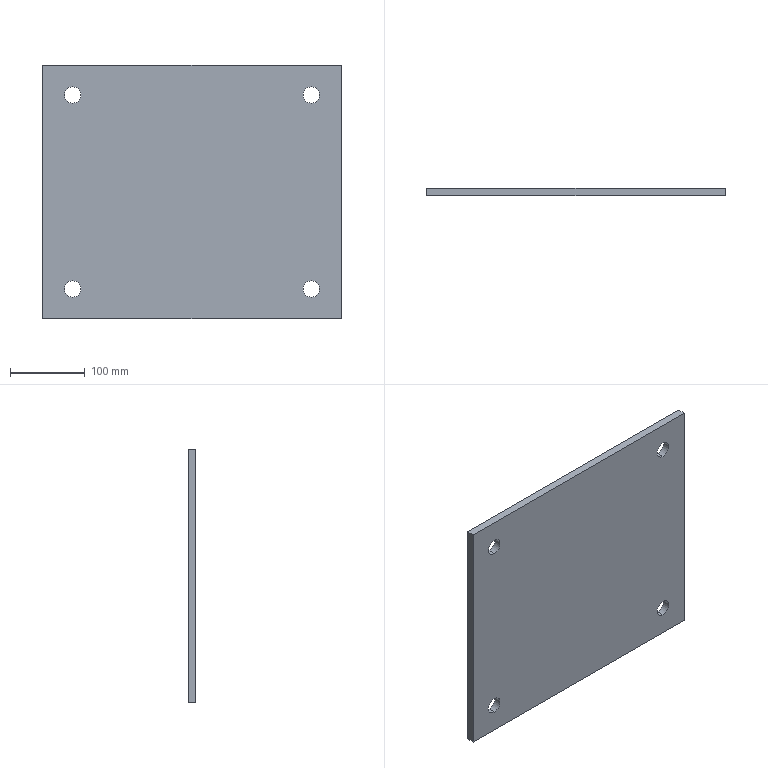Part | STEP file | 立柱Pad-中转釜 | 1 solid | 14 faces | box 400 x 10 x 340 mm | volume 1344795 mm3 | cylinder 8 | plane 6 | commonest cylinder face diameters 22 x8
STEP:
#1=CARTESIAN_POINT('',(0.,0.,0.));
#2=DIRECTION('',(0.,0.,1.));
#3=DIRECTION('',(1.,0.,0.));
#4=AXIS2_PLACEMENT_3D('',#1,#2,#3);
#5=CARTESIAN_POINT('',(160.,0.,-119.));
#6=VERTEX_POINT('',#5);
#7=CARTESIAN_POINT('',(160.,10.,-119.));
#8=VERTEX_POINT('',#7);
#9=CARTESIAN_POINT('',(160.,10.,-119.));
#10=DIRECTION('',(0.,1.,0.));
#11=VECTOR('',#10,1.);
#12=LINE('',#9,#11);
#13=CARTESIAN_POINT('',(160.,10.,-130.));
#14=DIRECTION('',(0.,1.,0.));
#15=DIRECTION('',(0.,0.,1.));
#16=AXIS2_PLACEMENT_3D('',#13,#14,#15);
#17=CYLINDRICAL_SURFACE('',#16,11.);
#18=CARTESIAN_POINT('',(6.283,0.));
#19=DIRECTION('',(0.,1.));
#20=VECTOR('',#19,1.);
#21=LINE('',#18,#20);
#22=(GEOMETRIC_REPRESENTATION_CONTEXT(2)PARAMETRIC_REPRESENTATION_CONTEXT()REPRESENTATION_CONTEXT('',''));
#23=DEFINITIONAL_REPRESENTATION('',(#21),#22);
#24=PCURVE('',#17,#23);
#25=CARTESIAN_POINT('',(160.,10.,-130.));
#26=DIRECTION('',(0.,1.,0.));
#27=DIRECTION('',(0.,0.,1.));
#28=AXIS2_PLACEMENT_3D('',#25,#26,#27);
#29=CYLINDRICAL_SURFACE('',#28,11.);
#30=CARTESIAN_POINT('',(0.,0.));
#31=DIRECTION('',(0.,1.));
#32=VECTOR('',#31,1.);
#33=LINE('',#30,#32);
#34=(GEOMETRIC_REPRESENTATION_CONTEXT(2)PARAMETRIC_REPRESENTATION_CONTEXT()REPRESENTATION_CONTEXT('',''));
#35=DEFINITIONAL_REPRESENTATION('',(#33),#34);
#36=PCURVE('',#29,#35);
#37=SURFACE_CURVE('',#12,(#24,#36),.PCURVE_S1.);
#38=EDGE_CURVE('',#6,#8,#37,.T.);
#39=ORIENTED_EDGE('',*,*,#38,.T.);
#40=CARTESIAN_POINT('',(160.,10.,-141.));
#41=VERTEX_POINT('',#40);
#42=CARTESIAN_POINT('',(160.,10.,-130.));
#43=DIRECTION('',(0.,1.,0.));
#44=DIRECTION('',(0.,0.,1.));
#45=AXIS2_PLACEMENT_3D('',#42,#43,#44);
#46=CIRCLE('',#45,11.);
#47=CARTESIAN_POINT('',(0.,0.));
#48=DIRECTION('',(1.,0.));
#49=VECTOR('',#48,1.);
#50=LINE('',#47,#49);
#51=(GEOMETRIC_REPRESENTATION_CONTEXT(2)PARAMETRIC_REPRESENTATION_CONTEXT()REPRESENTATION_CONTEXT('',''));
#52=DEFINITIONAL_REPRESENTATION('',(#50),#51);
#53=PCURVE('',#17,#52);
#54=CARTESIAN_POINT('',(0.,10.,0.));
#55=DIRECTION('',(0.,1.,0.));
#56=DIRECTION('',(0.,0.,1.));
#57=AXIS2_PLACEMENT_3D('',#54,#55,#56);
#58=PLANE('',#57);
#59=CARTESIAN_POINT('',(-130.,160.));
#60=DIRECTION('',(1.,0.));
#61=AXIS2_PLACEMENT_2D('',#59,#60);
#62=CIRCLE('',#61,11.);
#63=(GEOMETRIC_REPRESENTATION_CONTEXT(2)PARAMETRIC_REPRESENTATION_CONTEXT()REPRESENTATION_CONTEXT('',''));
#64=DEFINITIONAL_REPRESENTATION('',(#62),#63);
#65=PCURVE('',#58,#64);
#66=SURFACE_CURVE('',#46,(#53,#65),.PCURVE_S1.);
#67=EDGE_CURVE('',#41,#8,#66,.T.);
#68=ORIENTED_EDGE('',*,*,#67,.F.);
#69=CARTESIAN_POINT('',(160.,0.,-141.));
#70=VERTEX_POINT('',#69);
#71=CARTESIAN_POINT('',(160.,10.,-141.));
#72=DIRECTION('',(0.,1.,0.));
#73=VECTOR('',#72,1.);
#74=LINE('',#71,#73);
#75=CARTESIAN_POINT('',(3.142,0.));
#76=DIRECTION('',(0.,1.));
#77=VECTOR('',#76,1.);
#78=LINE('',#75,#77);
#79=(GEOMETRIC_REPRESENTATION_CONTEXT(2)PARAMETRIC_REPRESENTATION_CONTEXT()REPRESENTATION_CONTEXT('',''));
#80=DEFINITIONAL_REPRESENTATION('',(#78),#79);
#81=PCURVE('',#17,#80);
#82=CARTESIAN_POINT('',(3.142,0.));
#83=DIRECTION('',(0.,1.));
#84=VECTOR('',#83,1.);
#85=LINE('',#82,#84);
#86=(GEOMETRIC_REPRESENTATION_CONTEXT(2)PARAMETRIC_REPRESENTATION_CONTEXT()REPRESENTATION_CONTEXT('',''));
#87=DEFINITIONAL_REPRESENTATION('',(#85),#86);
#88=PCURVE('',#29,#87);
#89=SURFACE_CURVE('',#74,(#81,#88),.PCURVE_S1.);
#90=EDGE_CURVE('',#70,#41,#89,.T.);
#91=ORIENTED_EDGE('',*,*,#90,.F.);
#92=CARTESIAN_POINT('',(160.,0.,-130.));
#93=DIRECTION('',(0.,1.,0.));
#94=DIRECTION('',(0.,0.,1.));
#95=AXIS2_PLACEMENT_3D('',#92,#93,#94);
#96=CIRCLE('',#95,11.);
#97=CARTESIAN_POINT('',(0.,-10.));
#98=DIRECTION('',(1.,0.));
#99=VECTOR('',#98,1.);
#100=LINE('',#97,#99);
#101=(GEOMETRIC_REPRESENTATION_CONTEXT(2)PARAMETRIC_REPRESENTATION_CONTEXT()REPRESENTATION_CONTEXT('',''));
#102=DEFINITIONAL_REPRESENTATION('',(#100),#101);
#103=PCURVE('',#17,#102);
#104=CARTESIAN_POINT('',(0.,0.,0.));
#105=DIRECTION('',(0.,1.,0.));
#106=DIRECTION('',(0.,0.,1.));
#107=AXIS2_PLACEMENT_3D('',#104,#105,#106);
#108=PLANE('',#107);
#109=CARTESIAN_POINT('',(-130.,160.));
#110=DIRECTION('',(1.,0.));
#111=AXIS2_PLACEMENT_2D('',#109,#110);
#112=CIRCLE('',#111,11.);
#113=(GEOMETRIC_REPRESENTATION_CONTEXT(2)PARAMETRIC_REPRESENTATION_CONTEXT()REPRESENTATION_CONTEXT('',''));
#114=DEFINITIONAL_REPRESENTATION('',(#112),#113);
#115=PCURVE('',#108,#114);
#116=SURFACE_CURVE('',#96,(#103,#115),.PCURVE_S1.);
#117=EDGE_CURVE('',#70,#6,#116,.T.);
#118=ORIENTED_EDGE('',*,*,#117,.T.);
#119=EDGE_LOOP('',(#39,#68,#91,#118));
#120=FACE_BOUND('',#119,.F.);
#121=ADVANCED_FACE('',(#120),#17,.F.);
#122=CARTESIAN_POINT('',(160.,0.,141.));
#123=VERTEX_POINT('',#122);
#124=CARTESIAN_POINT('',(160.,10.,141.));
#125=VERTEX_POINT('',#124);
#126=CARTESIAN_POINT('',(160.,10.,141.));
#127=DIRECTION('',(0.,1.,0.));
#128=VECTOR('',#127,1.);
#129=LINE('',#126,#128);
#130=CARTESIAN_POINT('',(160.,10.,130.));
#131=DIRECTION('',(0.,1.,0.));
#132=DIRECTION('',(0.,0.,1.));
#133=AXIS2_PLACEMENT_3D('',#130,#131,#132);
#134=CYLINDRICAL_SURFACE('',#133,11.);
#135=CARTESIAN_POINT('',(6.283,0.));
#136=DIRECTION('',(0.,1.));
#137=VECTOR('',#136,1.);
#138=LINE('',#135,#137);
#139=(GEOMETRIC_REPRESENTATION_CONTEXT(2)PARAMETRIC_REPRESENTATION_CONTEXT()REPRESENTATION_CONTEXT('',''));
#140=DEFINITIONAL_REPRESENTATION('',(#138),#139);
#141=PCURVE('',#134,#140);
#142=CARTESIAN_POINT('',(160.,10.,130.));
#143=DIRECTION('',(0.,1.,0.));
#144=DIRECTION('',(0.,0.,1.));
#145=AXIS2_PLACEMENT_3D('',#142,#143,#144);
#146=CYLINDRICAL_SURFACE('',#145,11.);
#147=CARTESIAN_POINT('',(0.,0.));
#148=DIRECTION('',(0.,1.));
#149=VECTOR('',#148,1.);
#150=LINE('',#147,#149);
#151=(GEOMETRIC_REPRESENTATION_CONTEXT(2)PARAMETRIC_REPRESENTATION_CONTEXT()REPRESENTATION_CONTEXT('',''));
#152=DEFINITIONAL_REPRESENTATION('',(#150),#151);
#153=PCURVE('',#146,#152);
#154=SURFACE_CURVE('',#129,(#141,#153),.PCURVE_S1.);
#155=EDGE_CURVE('',#123,#125,#154,.T.);
#156=ORIENTED_EDGE('',*,*,#155,.T.);
#157=CARTESIAN_POINT('',(160.,10.,119.));
#158=VERTEX_POINT('',#157);
#159=CARTESIAN_POINT('',(160.,10.,130.));
#160=DIRECTION('',(0.,1.,0.));
#161=DIRECTION('',(0.,0.,1.));
#162=AXIS2_PLACEMENT_3D('',#159,#160,#161);
#163=CIRCLE('',#162,11.);
#164=CARTESIAN_POINT('',(0.,0.));
#165=DIRECTION('',(1.,0.));
#166=VECTOR('',#165,1.);
#167=LINE('',#164,#166);
#168=(GEOMETRIC_REPRESENTATION_CONTEXT(2)PARAMETRIC_REPRESENTATION_CONTEXT()REPRESENTATION_CONTEXT('',''));
#169=DEFINITIONAL_REPRESENTATION('',(#167),#168);
#170=PCURVE('',#134,#169);
#171=CARTESIAN_POINT('',(130.,160.));
#172=DIRECTION('',(1.,0.));
#173=AXIS2_PLACEMENT_2D('',#171,#172);
#174=CIRCLE('',#173,11.);
#175=(GEOMETRIC_REPRESENTATION_CONTEXT(2)PARAMETRIC_REPRESENTATION_CONTEXT()REPRESENTATION_CONTEXT('',''));
#176=DEFINITIONAL_REPRESENTATION('',(#174),#175);
#177=PCURVE('',#58,#176);
#178=SURFACE_CURVE('',#163,(#170,#177),.PCURVE_S1.);
#179=EDGE_CURVE('',#158,#125,#178,.T.);
#180=ORIENTED_EDGE('',*,*,#179,.F.);
#181=CARTESIAN_POINT('',(160.,0.,119.));
#182=VERTEX_POINT('',#181);
#183=CARTESIAN_POINT('',(160.,10.,119.));
#184=DIRECTION('',(0.,1.,0.));
#185=VECTOR('',#184,1.);
#186=LINE('',#183,#185);
#187=CARTESIAN_POINT('',(3.142,0.));
#188=DIRECTION('',(0.,1.));
#189=VECTOR('',#188,1.);
#190=LINE('',#187,#189);
#191=(GEOMETRIC_REPRESENTATION_CONTEXT(2)PARAMETRIC_REPRESENTATION_CONTEXT()REPRESENTATION_CONTEXT('',''));
#192=DEFINITIONAL_REPRESENTATION('',(#190),#191);
#193=PCURVE('',#134,#192);
#194=CARTESIAN_POINT('',(3.142,0.));
#195=DIRECTION('',(0.,1.));
#196=VECTOR('',#195,1.);
#197=LINE('',#194,#196);
#198=(GEOMETRIC_REPRESENTATION_CONTEXT(2)PARAMETRIC_REPRESENTATION_CONTEXT()REPRESENTATION_CONTEXT('',''));
#199=DEFINITIONAL_REPRESENTATION('',(#197),#198);
#200=PCURVE('',#146,#199);
#201=SURFACE_CURVE('',#186,(#193,#200),.PCURVE_S1.);
#202=EDGE_CURVE('',#182,#158,#201,.T.);
#203=ORIENTED_EDGE('',*,*,#202,.F.);
#204=CARTESIAN_POINT('',(160.,0.,130.));
#205=DIRECTION('',(0.,1.,0.));
#206=DIRECTION('',(0.,0.,1.));
#207=AXIS2_PLACEMENT_3D('',#204,#205,#206);
#208=CIRCLE('',#207,11.);
#209=CARTESIAN_POINT('',(0.,-10.));
#210=DIRECTION('',(1.,0.));
#211=VECTOR('',#210,1.);
#212=LINE('',#209,#211);
#213=(GEOMETRIC_REPRESENTATION_CONTEXT(2)PARAMETRIC_REPRESENTATION_CONTEXT()REPRESENTATION_CONTEXT('',''));
#214=DEFINITIONAL_REPRESENTATION('',(#212),#213);
#215=PCURVE('',#134,#214);
#216=CARTESIAN_POINT('',(130.,160.));
#217=DIRECTION('',(1.,0.));
#218=AXIS2_PLACEMENT_2D('',#216,#217);
#219=CIRCLE('',#218,11.);
#220=(GEOMETRIC_REPRESENTATION_CONTEXT(2)PARAMETRIC_REPRESENTATION_CONTEXT()REPRESENTATION_CONTEXT('',''));
#221=DEFINITIONAL_REPRESENTATION('',(#219),#220);
#222=PCURVE('',#108,#221);
#223=SURFACE_CURVE('',#208,(#215,#222),.PCURVE_S1.);
#224=EDGE_CURVE('',#182,#123,#223,.T.);
#225=ORIENTED_EDGE('',*,*,#224,.T.);
#226=EDGE_LOOP('',(#156,#180,#203,#225));
#227=FACE_BOUND('',#226,.F.);
#228=ADVANCED_FACE('',(#227),#134,.F.);
#229=CARTESIAN_POINT('',(-160.,0.,141.));
#230=VERTEX_POINT('',#229);
#231=CARTESIAN_POINT('',(-160.,10.,141.));
#232=VERTEX_POINT('',#231);
#233=CARTESIAN_POINT('',(-160.,10.,141.));
#234=DIRECTION('',(0.,1.,0.));
#235=VECTOR('',#234,1.);
#236=LINE('',#233,#235);
#237=CARTESIAN_POINT('',(-160.,10.,130.));
#238=DIRECTION('',(0.,1.,0.));
#239=DIRECTION('',(0.,0.,1.));
#240=AXIS2_PLACEMENT_3D('',#237,#238,#239);
#241=CYLINDRICAL_SURFACE('',#240,11.);
#242=CARTESIAN_POINT('',(6.283,0.));
#243=DIRECTION('',(0.,1.));
#244=VECTOR('',#243,1.);
#245=LINE('',#242,#244);
#246=(GEOMETRIC_REPRESENTATION_CONTEXT(2)PARAMETRIC_REPRESENTATION_CONTEXT()REPRESENTATION_CONTEXT('',''));
#247=DEFINITIONAL_REPRESENTATION('',(#245),#246);
#248=PCURVE('',#241,#247);
#249=CARTESIAN_POINT('',(-160.,10.,130.));
#250=DIRECTION('',(0.,1.,0.));
#251=DIRECTION('',(0.,0.,1.));
#252=AXIS2_PLACEMENT_3D('',#249,#250,#251);
#253=CYLINDRICAL_SURFACE('',#252,11.);
#254=CARTESIAN_POINT('',(0.,0.));
#255=DIRECTION('',(0.,1.));
#256=VECTOR('',#255,1.);
#257=LINE('',#254,#256);
#258=(GEOMETRIC_REPRESENTATION_CONTEXT(2)PARAMETRIC_REPRESENTATION_CONTEXT()REPRESENTATION_CONTEXT('',''));
#259=DEFINITIONAL_REPRESENTATION('',(#257),#258);
#260=PCURVE('',#253,#259);
#261=SURFACE_CURVE('',#236,(#248,#260),.PCURVE_S1.);
#262=EDGE_CURVE('',#230,#232,#261,.T.);
#263=ORIENTED_EDGE('',*,*,#262,.T.);
#264=CARTESIAN_POINT('',(-160.,10.,119.));
#265=VERTEX_POINT('',#264);
#266=CARTESIAN_POINT('',(-160.,10.,130.));
#267=DIRECTION('',(0.,1.,0.));
#268=DIRECTION('',(0.,0.,1.));
#269=AXIS2_PLACEMENT_3D('',#266,#267,#268);
#270=CIRCLE('',#269,11.);
#271=CARTESIAN_POINT('',(0.,0.));
#272=DIRECTION('',(1.,0.));
#273=VECTOR('',#272,1.);
#274=LINE('',#271,#273);
#275=(GEOMETRIC_REPRESENTATION_CONTEXT(2)PARAMETRIC_REPRESENTATION_CONTEXT()REPRESENTATION_CONTEXT('',''));
#276=DEFINITIONAL_REPRESENTATION('',(#274),#275);
#277=PCURVE('',#241,#276);
#278=CARTESIAN_POINT('',(130.,-160.));
#279=DIRECTION('',(1.,0.));
#280=AXIS2_PLACEMENT_2D('',#278,#279);
#281=CIRCLE('',#280,11.);
#282=(GEOMETRIC_REPRESENTATION_CONTEXT(2)PARAMETRIC_REPRESENTATION_CONTEXT()REPRESENTATION_CONTEXT('',''));
#283=DEFINITIONAL_REPRESENTATION('',(#281),#282);
#284=PCURVE('',#58,#283);
#285=SURFACE_CURVE('',#270,(#277,#284),.PCURVE_S1.);
#286=EDGE_CURVE('',#265,#232,#285,.T.);
#287=ORIENTED_EDGE('',*,*,#286,.F.);
#288=CARTESIAN_POINT('',(-160.,0.,119.));
#289=VERTEX_POINT('',#288);
#290=CARTESIAN_POINT('',(-160.,10.,119.));
#291=DIRECTION('',(0.,1.,0.));
#292=VECTOR('',#291,1.);
#293=LINE('',#290,#292);
#294=CARTESIAN_POINT('',(3.142,0.));
#295=DIRECTION('',(0.,1.));
#296=VECTOR('',#295,1.);
#297=LINE('',#294,#296);
#298=(GEOMETRIC_REPRESENTATION_CONTEXT(2)PARAMETRIC_REPRESENTATION_CONTEXT()REPRESENTATION_CONTEXT('',''));
#299=DEFINITIONAL_REPRESENTATION('',(#297),#298);
#300=PCURVE('',#241,#299);
#301=CARTESIAN_POINT('',(3.142,0.));
#302=DIRECTION('',(0.,1.));
#303=VECTOR('',#302,1.);
#304=LINE('',#301,#303);
#305=(GEOMETRIC_REPRESENTATION_CONTEXT(2)PARAMETRIC_REPRESENTATION_CONTEXT()REPRESENTATION_CONTEXT('',''));
#306=DEFINITIONAL_REPRESENTATION('',(#304),#305);
#307=PCURVE('',#253,#306);
#308=SURFACE_CURVE('',#293,(#300,#307),.PCURVE_S1.);
#309=EDGE_CURVE('',#289,#265,#308,.T.);
#310=ORIENTED_EDGE('',*,*,#309,.F.);
#311=CARTESIAN_POINT('',(-160.,0.,130.));
#312=DIRECTION('',(0.,1.,0.));
#313=DIRECTION('',(0.,0.,1.));
#314=AXIS2_PLACEMENT_3D('',#311,#312,#313);
#315=CIRCLE('',#314,11.);
#316=CARTESIAN_POINT('',(0.,-10.));
#317=DIRECTION('',(1.,0.));
#318=VECTOR('',#317,1.);
#319=LINE('',#316,#318);
#320=(GEOMETRIC_REPRESENTATION_CONTEXT(2)PARAMETRIC_REPRESENTATION_CONTEXT()REPRESENTATION_CONTEXT('',''));
#321=DEFINITIONAL_REPRESENTATION('',(#319),#320);
#322=PCURVE('',#241,#321);
#323=CARTESIAN_POINT('',(130.,-160.));
#324=DIRECTION('',(1.,0.));
#325=AXIS2_PLACEMENT_2D('',#323,#324);
#326=CIRCLE('',#325,11.);
#327=(GEOMETRIC_REPRESENTATION_CONTEXT(2)PARAMETRIC_REPRESENTATION_CONTEXT()REPRESENTATION_CONTEXT('',''));
#328=DEFINITIONAL_REPRESENTATION('',(#326),#327);
#329=PCURVE('',#108,#328);
#330=SURFACE_CURVE('',#315,(#322,#329),.PCURVE_S1.);
#331=EDGE_CURVE('',#289,#230,#330,.T.);
#332=ORIENTED_EDGE('',*,*,#331,.T.);
#333=EDGE_LOOP('',(#263,#287,#310,#332));
#334=FACE_BOUND('',#333,.F.);
#335=ADVANCED_FACE('',(#334),#241,.F.);
#336=CARTESIAN_POINT('',(-160.,0.,-119.));
#337=VERTEX_POINT('',#336);
#338=CARTESIAN_POINT('',(-160.,10.,-119.));
#339=VERTEX_POINT('',#338);
#340=CARTESIAN_POINT('',(-160.,10.,-119.));
#341=DIRECTION('',(0.,1.,0.));
#342=VECTOR('',#341,1.);
#343=LINE('',#340,#342);
#344=CARTESIAN_POINT('',(-160.,10.,-130.));
#345=DIRECTION('',(0.,1.,0.));
#346=DIRECTION('',(0.,0.,1.));
#347=AXIS2_PLACEMENT_3D('',#344,#345,#346);
#348=CYLINDRICAL_SURFACE('',#347,11.);
#349=CARTESIAN_POINT('',(6.283,0.));
#350=DIRECTION('',(0.,1.));
#351=VECTOR('',#350,1.);
#352=LINE('',#349,#351);
#353=(GEOMETRIC_REPRESENTATION_CONTEXT(2)PARAMETRIC_REPRESENTATION_CONTEXT()REPRESENTATION_CONTEXT('',''));
#354=DEFINITIONAL_REPRESENTATION('',(#352),#353);
#355=PCURVE('',#348,#354);
#356=CARTESIAN_POINT('',(-160.,10.,-130.));
#357=DIRECTION('',(0.,1.,0.));
#358=DIRECTION('',(0.,0.,1.));
#359=AXIS2_PLACEMENT_3D('',#356,#357,#358);
#360=CYLINDRICAL_SURFACE('',#359,11.);
#361=CARTESIAN_POINT('',(0.,0.));
#362=DIRECTION('',(0.,1.));
#363=VECTOR('',#362,1.);
#364=LINE('',#361,#363);
#365=(GEOMETRIC_REPRESENTATION_CONTEXT(2)PARAMETRIC_REPRESENTATION_CONTEXT()REPRESENTATION_CONTEXT('',''));
#366=DEFINITIONAL_REPRESENTATION('',(#364),#365);
#367=PCURVE('',#360,#366);
#368=SURFACE_CURVE('',#343,(#355,#367),.PCURVE_S1.);
#369=EDGE_CURVE('',#337,#339,#368,.T.);
#370=ORIENTED_EDGE('',*,*,#369,.T.);
#371=CARTESIAN_POINT('',(-160.,10.,-141.));
#372=VERTEX_POINT('',#371);
#373=CARTESIAN_POINT('',(-160.,10.,-130.));
#374=DIRECTION('',(0.,1.,0.));
#375=DIRECTION('',(0.,0.,1.));
#376=AXIS2_PLACEMENT_3D('',#373,#374,#375);
#377=CIRCLE('',#376,11.);
#378=CARTESIAN_POINT('',(0.,0.));
#379=DIRECTION('',(1.,0.));
#380=VECTOR('',#379,1.);
#381=LINE('',#378,#380);
#382=(GEOMETRIC_REPRESENTATION_CONTEXT(2)PARAMETRIC_REPRESENTATION_CONTEXT()REPRESENTATION_CONTEXT('',''));
#383=DEFINITIONAL_REPRESENTATION('',(#381),#382);
#384=PCURVE('',#348,#383);
#385=CARTESIAN_POINT('',(-130.,-160.));
#386=DIRECTION('',(1.,0.));
#387=AXIS2_PLACEMENT_2D('',#385,#386);
#388=CIRCLE('',#387,11.);
#389=(GEOMETRIC_REPRESENTATION_CONTEXT(2)PARAMETRIC_REPRESENTATION_CONTEXT()REPRESENTATION_CONTEXT('',''));
#390=DEFINITIONAL_REPRESENTATION('',(#388),#389);
#391=PCURVE('',#58,#390);
#392=SURFACE_CURVE('',#377,(#384,#391),.PCURVE_S1.);
#393=EDGE_CURVE('',#372,#339,#392,.T.);
#394=ORIENTED_EDGE('',*,*,#393,.F.);
#395=CARTESIAN_POINT('',(-160.,0.,-141.));
#396=VERTEX_POINT('',#395);
#397=CARTESIAN_POINT('',(-160.,10.,-141.));
#398=DIRECTION('',(0.,1.,0.));
#399=VECTOR('',#398,1.);
#400=LINE('',#397,#399);
#401=CARTESIAN_POINT('',(3.142,0.));
#402=DIRECTION('',(0.,1.));
#403=VECTOR('',#402,1.);
#404=LINE('',#401,#403);
#405=(GEOMETRIC_REPRESENTATION_CONTEXT(2)PARAMETRIC_REPRESENTATION_CONTEXT()REPRESENTATION_CONTEXT('',''));
#406=DEFINITIONAL_REPRESENTATION('',(#404),#405);
#407=PCURVE('',#348,#406);
#408=CARTESIAN_POINT('',(3.142,0.));
#409=DIRECTION('',(0.,1.));
#410=VECTOR('',#409,1.);
#411=LINE('',#408,#410);
#412=(GEOMETRIC_REPRESENTATION_CONTEXT(2)PARAMETRIC_REPRESENTATION_CONTEXT()REPRESENTATION_CONTEXT('',''));
#413=DEFINITIONAL_REPRESENTATION('',(#411),#412);
#414=PCURVE('',#360,#413);
#415=SURFACE_CURVE('',#400,(#407,#414),.PCURVE_S1.);
#416=EDGE_CURVE('',#396,#372,#415,.T.);
#417=ORIENTED_EDGE('',*,*,#416,.F.);
#418=CARTESIAN_POINT('',(-160.,0.,-130.));
#419=DIRECTION('',(0.,1.,0.));
#420=DIRECTION('',(0.,0.,1.));
#421=AXIS2_PLACEMENT_3D('',#418,#419,#420);
#422=CIRCLE('',#421,11.);
#423=CARTESIAN_POINT('',(0.,-10.));
#424=DIRECTION('',(1.,0.));
#425=VECTOR('',#424,1.);
#426=LINE('',#423,#425);
#427=(GEOMETRIC_REPRESENTATION_CONTEXT(2)PARAMETRIC_REPRESENTATION_CONTEXT()REPRESENTATION_CONTEXT('',''));
#428=DEFINITIONAL_REPRESENTATION('',(#426),#427);
#429=PCURVE('',#348,#428);
#430=CARTESIAN_POINT('',(-130.,-160.));
#431=DIRECTION('',(1.,0.));
#432=AXIS2_PLACEMENT_2D('',#430,#431);
#433=CIRCLE('',#432,11.);
#434=(GEOMETRIC_REPRESENTATION_CONTEXT(2)PARAMETRIC_REPRESENTATION_CONTEXT()REPRESENTATION_CONTEXT('',''));
#435=DEFINITIONAL_REPRESENTATION('',(#433),#434);
#436=PCURVE('',#108,#435);
#437=SURFACE_CURVE('',#422,(#429,#436),.PCURVE_S1.);
#438=EDGE_CURVE('',#396,#337,#437,.T.);
#439=ORIENTED_EDGE('',*,*,#438,.T.);
#440=EDGE_LOOP('',(#370,#394,#417,#439));
#441=FACE_BOUND('',#440,.F.);
#442=ADVANCED_FACE('',(#441),#348,.F.);
#443=CARTESIAN_POINT('',(200.,0.,170.));
#444=VERTEX_POINT('',#443);
#445=CARTESIAN_POINT('',(200.,0.,-170.));
#446=VERTEX_POINT('',#445);
#447=CARTESIAN_POINT('',(200.,0.,-170.));
#448=DIRECTION('',(0.,0.,-1.));
#449=VECTOR('',#448,1.);
#450=LINE('',#447,#449);
#451=CARTESIAN_POINT('',(200.,10.,-170.));
#452=DIRECTION('',(-1.,0.,0.));
#453=DIRECTION('',(0.,0.,1.));
#454=AXIS2_PLACEMENT_3D('',#451,#452,#453);
#455=PLANE('',#454);
#456=CARTESIAN_POINT('',(0.,-10.));
#457=DIRECTION('',(-1.,0.));
#458=VECTOR('',#457,1.);
#459=LINE('',#456,#458);
#460=(GEOMETRIC_REPRESENTATION_CONTEXT(2)PARAMETRIC_REPRESENTATION_CONTEXT()REPRESENTATION_CONTEXT('',''));
#461=DEFINITIONAL_REPRESENTATION('',(#459),#460);
#462=PCURVE('',#455,#461);
#463=CARTESIAN_POINT('',(-170.,200.));
#464=DIRECTION('',(-1.,0.));
#465=VECTOR('',#464,1.);
#466=LINE('',#463,#465);
#467=(GEOMETRIC_REPRESENTATION_CONTEXT(2)PARAMETRIC_REPRESENTATION_CONTEXT()REPRESENTATION_CONTEXT('',''));
#468=DEFINITIONAL_REPRESENTATION('',(#466),#467);
#469=PCURVE('',#108,#468);
#470=SURFACE_CURVE('',#450,(#462,#469),.PCURVE_S1.);
#471=EDGE_CURVE('',#444,#446,#470,.T.);
#472=ORIENTED_EDGE('',*,*,#471,.T.);
#473=CARTESIAN_POINT('',(200.,10.,-170.));
#474=VERTEX_POINT('',#473);
#475=CARTESIAN_POINT('',(200.,10.,-170.));
#476=DIRECTION('',(0.,-1.,0.));
#477=VECTOR('',#476,1.);
#478=LINE('',#475,#477);
#479=CARTESIAN_POINT('',(0.,0.));
#480=DIRECTION('',(0.,-1.));
#481=VECTOR('',#480,1.);
#482=LINE('',#479,#481);
#483=(GEOMETRIC_REPRESENTATION_CONTEXT(2)PARAMETRIC_REPRESENTATION_CONTEXT()REPRESENTATION_CONTEXT('',''));
#484=DEFINITIONAL_REPRESENTATION('',(#482),#483);
#485=PCURVE('',#455,#484);
#486=CARTESIAN_POINT('',(-200.,10.,-170.));
#487=DIRECTION('',(0.,0.,1.));
#488=DIRECTION('',(1.,0.,0.));
#489=AXIS2_PLACEMENT_3D('',#486,#487,#488);
#490=PLANE('',#489);
#491=CARTESIAN_POINT('',(400.,0.));
#492=DIRECTION('',(0.,-1.));
#493=VECTOR('',#492,1.);
#494=LINE('',#491,#493);
#495=(GEOMETRIC_REPRESENTATION_CONTEXT(2)PARAMETRIC_REPRESENTATION_CONTEXT()REPRESENTATION_CONTEXT('',''));
#496=DEFINITIONAL_REPRESENTATION('',(#494),#495);
#497=PCURVE('',#490,#496);
#498=SURFACE_CURVE('',#478,(#485,#497),.PCURVE_S1.);
#499=EDGE_CURVE('',#474,#446,#498,.T.);
#500=ORIENTED_EDGE('',*,*,#499,.F.);
#501=CARTESIAN_POINT('',(200.,10.,170.));
#502=VERTEX_POINT('',#501);
#503=CARTESIAN_POINT('',(200.,10.,-170.));
#504=DIRECTION('',(0.,0.,-1.));
#505=VECTOR('',#504,1.);
#506=LINE('',#503,#505);
#507=CARTESIAN_POINT('',(0.,0.));
#508=DIRECTION('',(-1.,0.));
#509=VECTOR('',#508,1.);
#510=LINE('',#507,#509);
#511=(GEOMETRIC_REPRESENTATION_CONTEXT(2)PARAMETRIC_REPRESENTATION_CONTEXT()REPRESENTATION_CONTEXT('',''));
#512=DEFINITIONAL_REPRESENTATION('',(#510),#511);
#513=PCURVE('',#455,#512);
#514=CARTESIAN_POINT('',(-170.,200.));
#515=DIRECTION('',(-1.,0.));
#516=VECTOR('',#515,1.);
#517=LINE('',#514,#516);
#518=(GEOMETRIC_REPRESENTATION_CONTEXT(2)PARAMETRIC_REPRESENTATION_CONTEXT()REPRESENTATION_CONTEXT('',''));
#519=DEFINITIONAL_REPRESENTATION('',(#517),#518);
#520=PCURVE('',#58,#519);
#521=SURFACE_CURVE('',#506,(#513,#520),.PCURVE_S1.);
#522=EDGE_CURVE('',#502,#474,#521,.T.);
#523=ORIENTED_EDGE('',*,*,#522,.F.);
#524=CARTESIAN_POINT('',(200.,10.,170.));
#525=DIRECTION('',(0.,-1.,0.));
#526=VECTOR('',#525,1.);
#527=LINE('',#524,#526);
#528=CARTESIAN_POINT('',(340.,0.));
#529=DIRECTION('',(0.,-1.));
#530=VECTOR('',#529,1.);
#531=LINE('',#528,#530);
#532=(GEOMETRIC_REPRESENTATION_CONTEXT(2)PARAMETRIC_REPRESENTATION_CONTEXT()REPRESENTATION_CONTEXT('',''));
#533=DEFINITIONAL_REPRESENTATION('',(#531),#532);
#534=PCURVE('',#455,#533);
#535=CARTESIAN_POINT('',(-200.,10.,170.));
#536=DIRECTION('',(0.,0.,-1.));
#537=DIRECTION('',(-1.,0.,0.));
#538=AXIS2_PLACEMENT_3D('',#535,#536,#537);
#539=PLANE('',#538);
#540=CARTESIAN_POINT('',(-400.,0.));
#541=DIRECTION('',(0.,-1.));
#542=VECTOR('',#541,1.);
#543=LINE('',#540,#542);
#544=(GEOMETRIC_REPRESENTATION_CONTEXT(2)PARAMETRIC_REPRESENTATION_CONTEXT()REPRESENTATION_CONTEXT('',''));
#545=DEFINITIONAL_REPRESENTATION('',(#543),#544);
#546=PCURVE('',#539,#545);
#547=SURFACE_CURVE('',#527,(#534,#546),.PCURVE_S1.);
#548=EDGE_CURVE('',#502,#444,#547,.T.);
#549=ORIENTED_EDGE('',*,*,#548,.T.);
#550=EDGE_LOOP('',(#472,#500,#523,#549));
#551=FACE_BOUND('',#550,.T.);
#552=ADVANCED_FACE('',(#551),#455,.F.);
#553=CARTESIAN_POINT('',(-200.,0.,-170.));
#554=VERTEX_POINT('',#553);
#555=CARTESIAN_POINT('',(-200.,0.,-170.));
#556=DIRECTION('',(-1.,0.,0.));
#557=VECTOR('',#556,1.);
#558=LINE('',#555,#557);
#559=CARTESIAN_POINT('',(0.,-10.));
#560=DIRECTION('',(-1.,0.));
#561=VECTOR('',#560,1.);
#562=LINE('',#559,#561);
#563=(GEOMETRIC_REPRESENTATION_CONTEXT(2)PARAMETRIC_REPRESENTATION_CONTEXT()REPRESENTATION_CONTEXT('',''));
#564=DEFINITIONAL_REPRESENTATION('',(#562),#563);
#565=PCURVE('',#490,#564);
#566=CARTESIAN_POINT('',(-170.,-200.));
#567=DIRECTION('',(0.,-1.));
#568=VECTOR('',#567,1.);
#569=LINE('',#566,#568);
#570=(GEOMETRIC_REPRESENTATION_CONTEXT(2)PARAMETRIC_REPRESENTATION_CONTEXT()REPRESENTATION_CONTEXT('',''));
#571=DEFINITIONAL_REPRESENTATION('',(#569),#570);
#572=PCURVE('',#108,#571);
#573=SURFACE_CURVE('',#558,(#565,#572),.PCURVE_S1.);
#574=EDGE_CURVE('',#446,#554,#573,.T.);
#575=ORIENTED_EDGE('',*,*,#574,.T.);
#576=CARTESIAN_POINT('',(-200.,10.,-170.));
#577=VERTEX_POINT('',#576);
#578=CARTESIAN_POINT('',(-200.,10.,-170.));
#579=DIRECTION('',(0.,-1.,0.));
#580=VECTOR('',#579,1.);
#581=LINE('',#578,#580);
#582=CARTESIAN_POINT('',(0.,0.));
#583=DIRECTION('',(0.,-1.));
#584=VECTOR('',#583,1.);
#585=LINE('',#582,#584);
#586=(GEOMETRIC_REPRESENTATION_CONTEXT(2)PARAMETRIC_REPRESENTATION_CONTEXT()REPRESENTATION_CONTEXT('',''));
#587=DEFINITIONAL_REPRESENTATION('',(#585),#586);
#588=PCURVE('',#490,#587);
#589=CARTESIAN_POINT('',(-200.,10.,-170.));
#590=DIRECTION('',(1.,0.,0.));
#591=DIRECTION('',(0.,0.,-1.));
#592=AXIS2_PLACEMENT_3D('',#589,#590,#591);
#593=PLANE('',#592);
#594=CARTESIAN_POINT('',(0.,0.));
#595=DIRECTION('',(0.,-1.));
#596=VECTOR('',#595,1.);
#597=LINE('',#594,#596);
#598=(GEOMETRIC_REPRESENTATION_CONTEXT(2)PARAMETRIC_REPRESENTATION_CONTEXT()REPRESENTATION_CONTEXT('',''));
#599=DEFINITIONAL_REPRESENTATION('',(#597),#598);
#600=PCURVE('',#593,#599);
#601=SURFACE_CURVE('',#581,(#588,#600),.PCURVE_S1.);
#602=EDGE_CURVE('',#577,#554,#601,.T.);
#603=ORIENTED_EDGE('',*,*,#602,.F.);
#604=CARTESIAN_POINT('',(-200.,10.,-170.));
#605=DIRECTION('',(-1.,0.,0.));
#606=VECTOR('',#605,1.);
#607=LINE('',#604,#606);
#608=CARTESIAN_POINT('',(0.,0.));
#609=DIRECTION('',(-1.,0.));
#610=VECTOR('',#609,1.);
#611=LINE('',#608,#610);
#612=(GEOMETRIC_REPRESENTATION_CONTEXT(2)PARAMETRIC_REPRESENTATION_CONTEXT()REPRESENTATION_CONTEXT('',''));
#613=DEFINITIONAL_REPRESENTATION('',(#611),#612);
#614=PCURVE('',#490,#613);
#615=CARTESIAN_POINT('',(-170.,-200.));
#616=DIRECTION('',(0.,-1.));
#617=VECTOR('',#616,1.);
#618=LINE('',#615,#617);
#619=(GEOMETRIC_REPRESENTATION_CONTEXT(2)PARAMETRIC_REPRESENTATION_CONTEXT()REPRESENTATION_CONTEXT('',''));
#620=DEFINITIONAL_REPRESENTATION('',(#618),#619);
#621=PCURVE('',#58,#620);
#622=SURFACE_CURVE('',#607,(#614,#621),.PCURVE_S1.);
#623=EDGE_CURVE('',#474,#577,#622,.T.);
#624=ORIENTED_EDGE('',*,*,#623,.F.);
#625=ORIENTED_EDGE('',*,*,#499,.T.);
#626=EDGE_LOOP('',(#575,#603,#624,#625));
#627=FACE_BOUND('',#626,.T.);
#628=ADVANCED_FACE('',(#627),#490,.F.);
#629=CARTESIAN_POINT('',(-200.,0.,170.));
#630=VERTEX_POINT('',#629);
#631=CARTESIAN_POINT('',(-200.,0.,-170.));
#632=DIRECTION('',(0.,0.,1.));
#633=VECTOR('',#632,1.);
#634=LINE('',#631,#633);
#635=CARTESIAN_POINT('',(0.,-10.));
#636=DIRECTION('',(-1.,0.));
#637=VECTOR('',#636,1.);
#638=LINE('',#635,#637);
#639=(GEOMETRIC_REPRESENTATION_CONTEXT(2)PARAMETRIC_REPRESENTATION_CONTEXT()REPRESENTATION_CONTEXT('',''));
#640=DEFINITIONAL_REPRESENTATION('',(#638),#639);
#641=PCURVE('',#593,#640);
#642=CARTESIAN_POINT('',(-170.,-200.));
#643=DIRECTION('',(1.,0.));
#644=VECTOR('',#643,1.);
#645=LINE('',#642,#644);
#646=(GEOMETRIC_REPRESENTATION_CONTEXT(2)PARAMETRIC_REPRESENTATION_CONTEXT()REPRESENTATION_CONTEXT('',''));
#647=DEFINITIONAL_REPRESENTATION('',(#645),#646);
#648=PCURVE('',#108,#647);
#649=SURFACE_CURVE('',#634,(#641,#648),.PCURVE_S1.);
#650=EDGE_CURVE('',#554,#630,#649,.T.);
#651=ORIENTED_EDGE('',*,*,#650,.T.);
#652=CARTESIAN_POINT('',(-200.,10.,170.));
#653=VERTEX_POINT('',#652);
#654=CARTESIAN_POINT('',(-200.,10.,170.));
#655=DIRECTION('',(0.,-1.,0.));
#656=VECTOR('',#655,1.);
#657=LINE('',#654,#656);
#658=CARTESIAN_POINT('',(-340.,0.));
#659=DIRECTION('',(0.,-1.));
#660=VECTOR('',#659,1.);
#661=LINE('',#658,#660);
#662=(GEOMETRIC_REPRESENTATION_CONTEXT(2)PARAMETRIC_REPRESENTATION_CONTEXT()REPRESENTATION_CONTEXT('',''));
#663=DEFINITIONAL_REPRESENTATION('',(#661),#662);
#664=PCURVE('',#593,#663);
#665=CARTESIAN_POINT('',(0.,0.));
#666=DIRECTION('',(0.,-1.));
#667=VECTOR('',#666,1.);
#668=LINE('',#665,#667);
#669=(GEOMETRIC_REPRESENTATION_CONTEXT(2)PARAMETRIC_REPRESENTATION_CONTEXT()REPRESENTATION_CONTEXT('',''));
#670=DEFINITIONAL_REPRESENTATION('',(#668),#669);
#671=PCURVE('',#539,#670);
#672=SURFACE_CURVE('',#657,(#664,#671),.PCURVE_S1.);
#673=EDGE_CURVE('',#653,#630,#672,.T.);
#674=ORIENTED_EDGE('',*,*,#673,.F.);
#675=CARTESIAN_POINT('',(-200.,10.,-170.));
#676=DIRECTION('',(0.,0.,1.));
#677=VECTOR('',#676,1.);
#678=LINE('',#675,#677);
#679=CARTESIAN_POINT('',(0.,0.));
#680=DIRECTION('',(-1.,0.));
#681=VECTOR('',#680,1.);
#682=LINE('',#679,#681);
#683=(GEOMETRIC_REPRESENTATION_CONTEXT(2)PARAMETRIC_REPRESENTATION_CONTEXT()REPRESENTATION_CONTEXT('',''));
#684=DEFINITIONAL_REPRESENTATION('',(#682),#683);
#685=PCURVE('',#593,#684);
#686=CARTESIAN_POINT('',(-170.,-200.));
#687=DIRECTION('',(1.,0.));
#688=VECTOR('',#687,1.);
#689=LINE('',#686,#688);
#690=(GEOMETRIC_REPRESENTATION_CONTEXT(2)PARAMETRIC_REPRESENTATION_CONTEXT()REPRESENTATION_CONTEXT('',''));
#691=DEFINITIONAL_REPRESENTATION('',(#689),#690);
#692=PCURVE('',#58,#691);
#693=SURFACE_CURVE('',#678,(#685,#692),.PCURVE_S1.);
#694=EDGE_CURVE('',#577,#653,#693,.T.);
#695=ORIENTED_EDGE('',*,*,#694,.F.);
#696=ORIENTED_EDGE('',*,*,#602,.T.);
#697=EDGE_LOOP('',(#651,#674,#695,#696));
#698=FACE_BOUND('',#697,.T.);
#699=ADVANCED_FACE('',(#698),#593,.F.);
#700=CARTESIAN_POINT('',(-200.,0.,170.));
#701=DIRECTION('',(1.,0.,0.));
#702=VECTOR('',#701,1.);
#703=LINE('',#700,#702);
#704=CARTESIAN_POINT('',(0.,-10.));
#705=DIRECTION('',(-1.,0.));
#706=VECTOR('',#705,1.);
#707=LINE('',#704,#706);
#708=(GEOMETRIC_REPRESENTATION_CONTEXT(2)PARAMETRIC_REPRESENTATION_CONTEXT()REPRESENTATION_CONTEXT('',''));
#709=DEFINITIONAL_REPRESENTATION('',(#707),#708);
#710=PCURVE('',#539,#709);
#711=CARTESIAN_POINT('',(170.,-200.));
#712=DIRECTION('',(0.,1.));
#713=VECTOR('',#712,1.);
#714=LINE('',#711,#713);
#715=(GEOMETRIC_REPRESENTATION_CONTEXT(2)PARAMETRIC_REPRESENTATION_CONTEXT()REPRESENTATION_CONTEXT('',''));
#716=DEFINITIONAL_REPRESENTATION('',(#714),#715);
#717=PCURVE('',#108,#716);
#718=SURFACE_CURVE('',#703,(#710,#717),.PCURVE_S1.);
#719=EDGE_CURVE('',#630,#444,#718,.T.);
#720=ORIENTED_EDGE('',*,*,#719,.T.);
#721=ORIENTED_EDGE('',*,*,#548,.F.);
#722=CARTESIAN_POINT('',(-200.,10.,170.));
#723=DIRECTION('',(1.,0.,0.));
#724=VECTOR('',#723,1.);
#725=LINE('',#722,#724);
#726=CARTESIAN_POINT('',(0.,0.));
#727=DIRECTION('',(-1.,0.));
#728=VECTOR('',#727,1.);
#729=LINE('',#726,#728);
#730=(GEOMETRIC_REPRESENTATION_CONTEXT(2)PARAMETRIC_REPRESENTATION_CONTEXT()REPRESENTATION_CONTEXT('',''));
#731=DEFINITIONAL_REPRESENTATION('',(#729),#730);
#732=PCURVE('',#539,#731);
#733=CARTESIAN_POINT('',(170.,-200.));
#734=DIRECTION('',(0.,1.));
#735=VECTOR('',#734,1.);
#736=LINE('',#733,#735);
#737=(GEOMETRIC_REPRESENTATION_CONTEXT(2)PARAMETRIC_REPRESENTATION_CONTEXT()REPRESENTATION_CONTEXT('',''));
#738=DEFINITIONAL_REPRESENTATION('',(#736),#737);
#739=PCURVE('',#58,#738);
#740=SURFACE_CURVE('',#725,(#732,#739),.PCURVE_S1.);
#741=EDGE_CURVE('',#653,#502,#740,.T.);
#742=ORIENTED_EDGE('',*,*,#741,.F.);
#743=ORIENTED_EDGE('',*,*,#673,.T.);
#744=EDGE_LOOP('',(#720,#721,#742,#743));
#745=FACE_BOUND('',#744,.T.);
#746=ADVANCED_FACE('',(#745),#539,.F.);
#747=CARTESIAN_POINT('',(160.,10.,-130.));
#748=DIRECTION('',(0.,1.,0.));
#749=DIRECTION('',(0.,0.,1.));
#750=AXIS2_PLACEMENT_3D('',#747,#748,#749);
#751=CIRCLE('',#750,11.);
#752=CARTESIAN_POINT('',(-130.,160.));
#753=DIRECTION('',(1.,0.));
#754=AXIS2_PLACEMENT_2D('',#752,#753);
#755=CIRCLE('',#754,11.);
#756=(GEOMETRIC_REPRESENTATION_CONTEXT(2)PARAMETRIC_REPRESENTATION_CONTEXT()REPRESENTATION_CONTEXT('',''));
#757=DEFINITIONAL_REPRESENTATION('',(#755),#756);
#758=PCURVE('',#58,#757);
#759=CARTESIAN_POINT('',(0.,0.));
#760=DIRECTION('',(1.,0.));
#761=VECTOR('',#760,1.);
#762=LINE('',#759,#761);
#763=(GEOMETRIC_REPRESENTATION_CONTEXT(2)PARAMETRIC_REPRESENTATION_CONTEXT()REPRESENTATION_CONTEXT('',''));
#764=DEFINITIONAL_REPRESENTATION('',(#762),#763);
#765=PCURVE('',#29,#764);
#766=SURFACE_CURVE('',#751,(#758,#765),.PCURVE_S1.);
#767=EDGE_CURVE('',#8,#41,#766,.T.);
#768=ORIENTED_EDGE('',*,*,#767,.F.);
#769=ORIENTED_EDGE('',*,*,#67,.F.);
#770=EDGE_LOOP('',(#768,#769));
#771=FACE_BOUND('',#770,.T.);
#772=CARTESIAN_POINT('',(160.,10.,130.));
#773=DIRECTION('',(0.,1.,0.));
#774=DIRECTION('',(0.,0.,1.));
#775=AXIS2_PLACEMENT_3D('',#772,#773,#774);
#776=CIRCLE('',#775,11.);
#777=CARTESIAN_POINT('',(130.,160.));
#778=DIRECTION('',(1.,0.));
#779=AXIS2_PLACEMENT_2D('',#777,#778);
#780=CIRCLE('',#779,11.);
#781=(GEOMETRIC_REPRESENTATION_CONTEXT(2)PARAMETRIC_REPRESENTATION_CONTEXT()REPRESENTATION_CONTEXT('',''));
#782=DEFINITIONAL_REPRESENTATION('',(#780),#781);
#783=PCURVE('',#58,#782);
#784=CARTESIAN_POINT('',(0.,0.));
#785=DIRECTION('',(1.,0.));
#786=VECTOR('',#785,1.);
#787=LINE('',#784,#786);
#788=(GEOMETRIC_REPRESENTATION_CONTEXT(2)PARAMETRIC_REPRESENTATION_CONTEXT()REPRESENTATION_CONTEXT('',''));
#789=DEFINITIONAL_REPRESENTATION('',(#787),#788);
#790=PCURVE('',#146,#789);
#791=SURFACE_CURVE('',#776,(#783,#790),.PCURVE_S1.);
#792=EDGE_CURVE('',#125,#158,#791,.T.);
#793=ORIENTED_EDGE('',*,*,#792,.F.);
#794=ORIENTED_EDGE('',*,*,#179,.F.);
#795=EDGE_LOOP('',(#793,#794));
#796=FACE_BOUND('',#795,.T.);
#797=CARTESIAN_POINT('',(-160.,10.,130.));
#798=DIRECTION('',(0.,1.,0.));
#799=DIRECTION('',(0.,0.,1.));
#800=AXIS2_PLACEMENT_3D('',#797,#798,#799);
#801=CIRCLE('',#800,11.);
#802=CARTESIAN_POINT('',(130.,-160.));
#803=DIRECTION('',(1.,0.));
#804=AXIS2_PLACEMENT_2D('',#802,#803);
#805=CIRCLE('',#804,11.);
#806=(GEOMETRIC_REPRESENTATION_CONTEXT(2)PARAMETRIC_REPRESENTATION_CONTEXT()REPRESENTATION_CONTEXT('',''));
#807=DEFINITIONAL_REPRESENTATION('',(#805),#806);
#808=PCURVE('',#58,#807);
#809=CARTESIAN_POINT('',(0.,0.));
#810=DIRECTION('',(1.,0.));
#811=VECTOR('',#810,1.);
#812=LINE('',#809,#811);
#813=(GEOMETRIC_REPRESENTATION_CONTEXT(2)PARAMETRIC_REPRESENTATION_CONTEXT()REPRESENTATION_CONTEXT('',''));
#814=DEFINITIONAL_REPRESENTATION('',(#812),#813);
#815=PCURVE('',#253,#814);
#816=SURFACE_CURVE('',#801,(#808,#815),.PCURVE_S1.);
#817=EDGE_CURVE('',#232,#265,#816,.T.);
#818=ORIENTED_EDGE('',*,*,#817,.F.);
#819=ORIENTED_EDGE('',*,*,#286,.F.);
#820=EDGE_LOOP('',(#818,#819));
#821=FACE_BOUND('',#820,.T.);
#822=CARTESIAN_POINT('',(-160.,10.,-130.));
#823=DIRECTION('',(0.,1.,0.));
#824=DIRECTION('',(0.,0.,1.));
#825=AXIS2_PLACEMENT_3D('',#822,#823,#824);
#826=CIRCLE('',#825,11.);
#827=CARTESIAN_POINT('',(-130.,-160.));
#828=DIRECTION('',(1.,0.));
#829=AXIS2_PLACEMENT_2D('',#827,#828);
#830=CIRCLE('',#829,11.);
#831=(GEOMETRIC_REPRESENTATION_CONTEXT(2)PARAMETRIC_REPRESENTATION_CONTEXT()REPRESENTATION_CONTEXT('',''));
#832=DEFINITIONAL_REPRESENTATION('',(#830),#831);
#833=PCURVE('',#58,#832);
#834=CARTESIAN_POINT('',(0.,0.));
#835=DIRECTION('',(1.,0.));
#836=VECTOR('',#835,1.);
#837=LINE('',#834,#836);
#838=(GEOMETRIC_REPRESENTATION_CONTEXT(2)PARAMETRIC_REPRESENTATION_CONTEXT()REPRESENTATION_CONTEXT('',''));
#839=DEFINITIONAL_REPRESENTATION('',(#837),#838);
#840=PCURVE('',#360,#839);
#841=SURFACE_CURVE('',#826,(#833,#840),.PCURVE_S1.);
#842=EDGE_CURVE('',#339,#372,#841,.T.);
#843=ORIENTED_EDGE('',*,*,#842,.F.);
#844=ORIENTED_EDGE('',*,*,#393,.F.);
#845=EDGE_LOOP('',(#843,#844));
#846=FACE_BOUND('',#845,.T.);
#847=ORIENTED_EDGE('',*,*,#522,.T.);
#848=ORIENTED_EDGE('',*,*,#623,.T.);
#849=ORIENTED_EDGE('',*,*,#694,.T.);
#850=ORIENTED_EDGE('',*,*,#741,.T.);
#851=EDGE_LOOP('',(#847,#848,#849,#850));
#852=FACE_BOUND('',#851,.T.);
#853=ADVANCED_FACE('',(#771,#796,#821,#846,#852),#58,.T.);
#854=CARTESIAN_POINT('',(160.,0.,-130.));
#855=DIRECTION('',(0.,1.,0.));
#856=DIRECTION('',(0.,0.,1.));
#857=AXIS2_PLACEMENT_3D('',#854,#855,#856);
#858=CIRCLE('',#857,11.);
#859=CARTESIAN_POINT('',(-130.,160.));
#860=DIRECTION('',(1.,0.));
#861=AXIS2_PLACEMENT_2D('',#859,#860);
#862=CIRCLE('',#861,11.);
#863=(GEOMETRIC_REPRESENTATION_CONTEXT(2)PARAMETRIC_REPRESENTATION_CONTEXT()REPRESENTATION_CONTEXT('',''));
#864=DEFINITIONAL_REPRESENTATION('',(#862),#863);
#865=PCURVE('',#108,#864);
#866=CARTESIAN_POINT('',(0.,-10.));
#867=DIRECTION('',(1.,0.));
#868=VECTOR('',#867,1.);
#869=LINE('',#866,#868);
#870=(GEOMETRIC_REPRESENTATION_CONTEXT(2)PARAMETRIC_REPRESENTATION_CONTEXT()REPRESENTATION_CONTEXT('',''));
#871=DEFINITIONAL_REPRESENTATION('',(#869),#870);
#872=PCURVE('',#29,#871);
#873=SURFACE_CURVE('',#858,(#865,#872),.PCURVE_S1.);
#874=EDGE_CURVE('',#6,#70,#873,.T.);
#875=ORIENTED_EDGE('',*,*,#874,.T.);
#876=ORIENTED_EDGE('',*,*,#117,.T.);
#877=EDGE_LOOP('',(#875,#876));
#878=FACE_BOUND('',#877,.T.);
#879=CARTESIAN_POINT('',(160.,0.,130.));
#880=DIRECTION('',(0.,1.,0.));
#881=DIRECTION('',(0.,0.,1.));
#882=AXIS2_PLACEMENT_3D('',#879,#880,#881);
#883=CIRCLE('',#882,11.);
#884=CARTESIAN_POINT('',(130.,160.));
#885=DIRECTION('',(1.,0.));
#886=AXIS2_PLACEMENT_2D('',#884,#885);
#887=CIRCLE('',#886,11.);
#888=(GEOMETRIC_REPRESENTATION_CONTEXT(2)PARAMETRIC_REPRESENTATION_CONTEXT()REPRESENTATION_CONTEXT('',''));
#889=DEFINITIONAL_REPRESENTATION('',(#887),#888);
#890=PCURVE('',#108,#889);
#891=CARTESIAN_POINT('',(0.,-10.));
#892=DIRECTION('',(1.,0.));
#893=VECTOR('',#892,1.);
#894=LINE('',#891,#893);
#895=(GEOMETRIC_REPRESENTATION_CONTEXT(2)PARAMETRIC_REPRESENTATION_CONTEXT()REPRESENTATION_CONTEXT('',''));
#896=DEFINITIONAL_REPRESENTATION('',(#894),#895);
#897=PCURVE('',#146,#896);
#898=SURFACE_CURVE('',#883,(#890,#897),.PCURVE_S1.);
#899=EDGE_CURVE('',#123,#182,#898,.T.);
#900=ORIENTED_EDGE('',*,*,#899,.T.);
#901=ORIENTED_EDGE('',*,*,#224,.T.);
#902=EDGE_LOOP('',(#900,#901));
#903=FACE_BOUND('',#902,.T.);
#904=CARTESIAN_POINT('',(-160.,0.,130.));
#905=DIRECTION('',(0.,1.,0.));
#906=DIRECTION('',(0.,0.,1.));
#907=AXIS2_PLACEMENT_3D('',#904,#905,#906);
#908=CIRCLE('',#907,11.);
#909=CARTESIAN_POINT('',(130.,-160.));
#910=DIRECTION('',(1.,0.));
#911=AXIS2_PLACEMENT_2D('',#909,#910);
#912=CIRCLE('',#911,11.);
#913=(GEOMETRIC_REPRESENTATION_CONTEXT(2)PARAMETRIC_REPRESENTATION_CONTEXT()REPRESENTATION_CONTEXT('',''));
#914=DEFINITIONAL_REPRESENTATION('',(#912),#913);
#915=PCURVE('',#108,#914);
#916=CARTESIAN_POINT('',(0.,-10.));
#917=DIRECTION('',(1.,0.));
#918=VECTOR('',#917,1.);
#919=LINE('',#916,#918);
#920=(GEOMETRIC_REPRESENTATION_CONTEXT(2)PARAMETRIC_REPRESENTATION_CONTEXT()REPRESENTATION_CONTEXT('',''));
#921=DEFINITIONAL_REPRESENTATION('',(#919),#920);
#922=PCURVE('',#253,#921);
#923=SURFACE_CURVE('',#908,(#915,#922),.PCURVE_S1.);
#924=EDGE_CURVE('',#230,#289,#923,.T.);
#925=ORIENTED_EDGE('',*,*,#924,.T.);
#926=ORIENTED_EDGE('',*,*,#331,.T.);
#927=EDGE_LOOP('',(#925,#926));
#928=FACE_BOUND('',#927,.T.);
#929=CARTESIAN_POINT('',(-160.,0.,-130.));
#930=DIRECTION('',(0.,1.,0.));
#931=DIRECTION('',(0.,0.,1.));
#932=AXIS2_PLACEMENT_3D('',#929,#930,#931);
#933=CIRCLE('',#932,11.);
#934=CARTESIAN_POINT('',(-130.,-160.));
#935=DIRECTION('',(1.,0.));
#936=AXIS2_PLACEMENT_2D('',#934,#935);
#937=CIRCLE('',#936,11.);
#938=(GEOMETRIC_REPRESENTATION_CONTEXT(2)PARAMETRIC_REPRESENTATION_CONTEXT()REPRESENTATION_CONTEXT('',''));
#939=DEFINITIONAL_REPRESENTATION('',(#937),#938);
#940=PCURVE('',#108,#939);
#941=CARTESIAN_POINT('',(0.,-10.));
#942=DIRECTION('',(1.,0.));
#943=VECTOR('',#942,1.);
#944=LINE('',#941,#943);
#945=(GEOMETRIC_REPRESENTATION_CONTEXT(2)PARAMETRIC_REPRESENTATION_CONTEXT()REPRESENTATION_CONTEXT('',''));
#946=DEFINITIONAL_REPRESENTATION('',(#944),#945);
#947=PCURVE('',#360,#946);
#948=SURFACE_CURVE('',#933,(#940,#947),.PCURVE_S1.);
#949=EDGE_CURVE('',#337,#396,#948,.T.);
#950=ORIENTED_EDGE('',*,*,#949,.T.);
#951=ORIENTED_EDGE('',*,*,#438,.T.);
#952=EDGE_LOOP('',(#950,#951));
#953=FACE_BOUND('',#952,.T.);
#954=ORIENTED_EDGE('',*,*,#471,.F.);
#955=ORIENTED_EDGE('',*,*,#719,.F.);
#956=ORIENTED_EDGE('',*,*,#650,.F.);
#957=ORIENTED_EDGE('',*,*,#574,.F.);
#958=EDGE_LOOP('',(#954,#955,#956,#957));
#959=FACE_BOUND('',#958,.T.);
#960=ADVANCED_FACE('',(#878,#903,#928,#953,#959),#108,.F.);
#961=ORIENTED_EDGE('',*,*,#842,.F.);
#962=ORIENTED_EDGE('',*,*,#369,.F.);
#963=ORIENTED_EDGE('',*,*,#949,.T.);
#964=ORIENTED_EDGE('',*,*,#416,.T.);
#965=EDGE_LOOP('',(#961,#962,#963,#964));
#966=FACE_BOUND('',#965,.F.);
#967=ADVANCED_FACE('',(#966),#360,.F.);
#968=ORIENTED_EDGE('',*,*,#817,.F.);
#969=ORIENTED_EDGE('',*,*,#262,.F.);
#970=ORIENTED_EDGE('',*,*,#924,.T.);
#971=ORIENTED_EDGE('',*,*,#309,.T.);
#972=EDGE_LOOP('',(#968,#969,#970,#971));
#973=FACE_BOUND('',#972,.F.);
#974=ADVANCED_FACE('',(#973),#253,.F.);
#975=ORIENTED_EDGE('',*,*,#792,.F.);
#976=ORIENTED_EDGE('',*,*,#155,.F.);
#977=ORIENTED_EDGE('',*,*,#899,.T.);
#978=ORIENTED_EDGE('',*,*,#202,.T.);
#979=EDGE_LOOP('',(#975,#976,#977,#978));
#980=FACE_BOUND('',#979,.F.);
#981=ADVANCED_FACE('',(#980),#146,.F.);
#982=ORIENTED_EDGE('',*,*,#767,.F.);
#983=ORIENTED_EDGE('',*,*,#38,.F.);
#984=ORIENTED_EDGE('',*,*,#874,.T.);
#985=ORIENTED_EDGE('',*,*,#90,.T.);
#986=EDGE_LOOP('',(#982,#983,#984,#985));
#987=FACE_BOUND('',#986,.F.);
#988=ADVANCED_FACE('',(#987),#29,.F.);
#989=CLOSED_SHELL('',(#121,#228,#335,#442,#552,#628,#699,#746,#853,#960,#967,#974,#981,#988));
#990=MANIFOLD_SOLID_BREP('',#989);
#991=(LENGTH_UNIT()NAMED_UNIT(*)SI_UNIT(.MILLI.,.METRE.));
#992=UNCERTAINTY_MEASURE_WITH_UNIT(LENGTH_MEASURE(0.0000001),#991,'','');
#993=(NAMED_UNIT(*)PLANE_ANGLE_UNIT()SI_UNIT($,.RADIAN.));
#994=(NAMED_UNIT(*)SI_UNIT($,.STERADIAN.)SOLID_ANGLE_UNIT());
#995=(GEOMETRIC_REPRESENTATION_CONTEXT(3)GLOBAL_UNCERTAINTY_ASSIGNED_CONTEXT((#992))GLOBAL_UNIT_ASSIGNED_CONTEXT((#991,#993,#994))REPRESENTATION_CONTEXT('',''));
#996=ADVANCED_BREP_SHAPE_REPRESENTATION('',(#4,#990),#995);